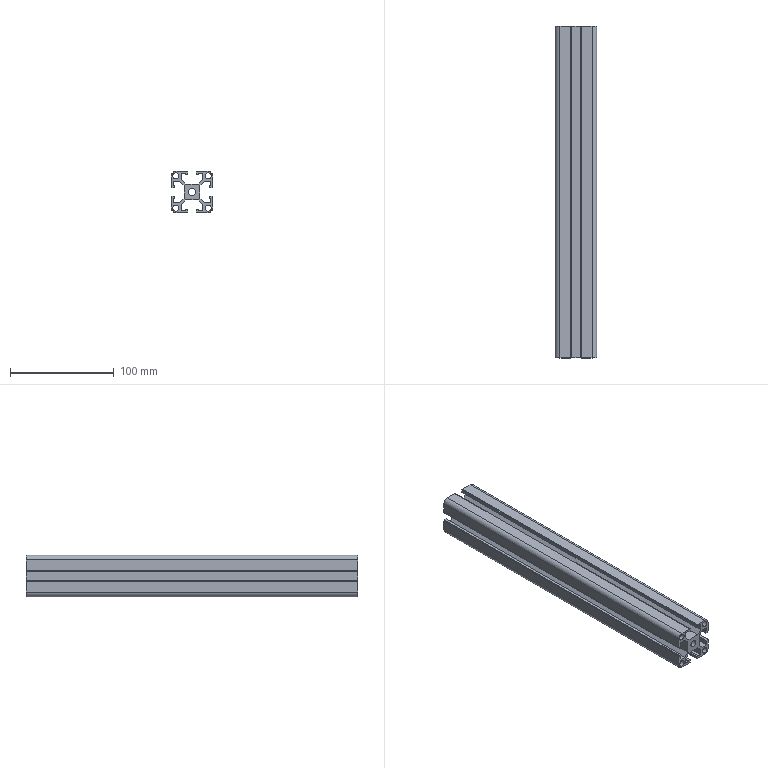Part | SolidWorks | features WeldMemberFeat 1, WeldmentFeature 1 | 1 solid | 92 faces | box 40 x 320 x 40 mm | volume 193550 mm3 | plane 78 | cylinder 14 | commonest cylinder face diameters 6 x8 9 x4 6.8 x2